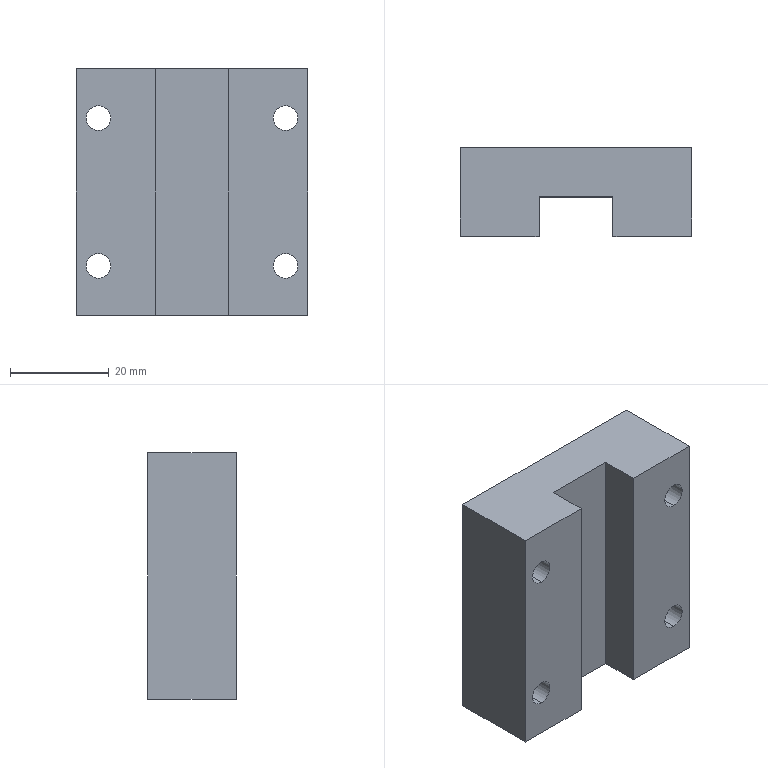Part | 1 solid | 18 faces | box 47 x 18 x 50 mm | volume 34886 mm3 | plane 10 | cylinder 8 | commonest cylinder face diameters 5 x8
STEP:
#1=CARTESIAN_POINT('',(-19.,-9.,37.5));
#2=VERTEX_POINT('',#1);
#3=CARTESIAN_POINT('',(-19.,-9.,42.5));
#4=VERTEX_POINT('',#3);
#5=CARTESIAN_POINT('',(-19.,-9.,40.));
#6=DIRECTION('',(0.,1.,0.));
#7=DIRECTION('',(-1.,0.,0.));
#8=AXIS2_PLACEMENT_3D('',#5,#6,#7);
#9=CIRCLE('',#8,2.5);
#10=EDGE_CURVE('',#2,#4,#9,.T.);
#11=ORIENTED_EDGE('',*,*,#10,.F.);
#12=CARTESIAN_POINT('',(-19.,9.,37.5));
#13=VERTEX_POINT('',#12);
#14=CARTESIAN_POINT('',(-19.,-41.,37.5));
#15=DIRECTION('',(0.,1.,0.));
#16=VECTOR('',#15,1000.);
#17=LINE('',#14,#16);
#18=EDGE_CURVE('',#2,#13,#17,.T.);
#19=ORIENTED_EDGE('',*,*,#18,.T.);
#20=CARTESIAN_POINT('',(-19.,9.,42.5));
#21=VERTEX_POINT('',#20);
#22=CARTESIAN_POINT('',(-19.,9.,40.));
#23=DIRECTION('',(0.,1.,0.));
#24=DIRECTION('',(0.,0.,1.));
#25=AXIS2_PLACEMENT_3D('',#22,#23,#24);
#26=CIRCLE('',#25,2.5);
#27=EDGE_CURVE('',#13,#21,#26,.T.);
#28=ORIENTED_EDGE('',*,*,#27,.T.);
#29=CARTESIAN_POINT('',(-19.,-41.,42.5));
#30=DIRECTION('',(0.,1.,0.));
#31=VECTOR('',#30,1000.);
#32=LINE('',#29,#31);
#33=EDGE_CURVE('',#4,#21,#32,.T.);
#34=ORIENTED_EDGE('',*,*,#33,.F.);
#35=EDGE_LOOP('',(#11,#19,#28,#34));
#36=FACE_OUTER_BOUND('',#35,.T.);
#37=CARTESIAN_POINT('',(-19.,-41.,40.));
#38=DIRECTION('',(0.,1.,0.));
#39=DIRECTION('',(0.,0.,1.));
#40=AXIS2_PLACEMENT_3D('',#37,#38,#39);
#41=CYLINDRICAL_SURFACE('',#40,2.5);
#42=ADVANCED_FACE('',(#36),#41,.F.);
#43=CARTESIAN_POINT('',(-19.,-9.,7.5));
#44=VERTEX_POINT('',#43);
#45=CARTESIAN_POINT('',(-19.,-9.,12.5));
#46=VERTEX_POINT('',#45);
#47=CARTESIAN_POINT('',(-19.,-9.,10.));
#48=DIRECTION('',(0.,1.,0.));
#49=DIRECTION('',(-1.,0.,0.));
#50=AXIS2_PLACEMENT_3D('',#47,#48,#49);
#51=CIRCLE('',#50,2.5);
#52=EDGE_CURVE('',#44,#46,#51,.T.);
#53=ORIENTED_EDGE('',*,*,#52,.F.);
#54=CARTESIAN_POINT('',(-19.,9.,7.5));
#55=VERTEX_POINT('',#54);
#56=CARTESIAN_POINT('',(-19.,-41.,7.5));
#57=DIRECTION('',(0.,1.,0.));
#58=VECTOR('',#57,1000.);
#59=LINE('',#56,#58);
#60=EDGE_CURVE('',#44,#55,#59,.T.);
#61=ORIENTED_EDGE('',*,*,#60,.T.);
#62=CARTESIAN_POINT('',(-19.,9.,12.5));
#63=VERTEX_POINT('',#62);
#64=CARTESIAN_POINT('',(-19.,9.,10.));
#65=DIRECTION('',(0.,1.,0.));
#66=DIRECTION('',(0.,0.,1.));
#67=AXIS2_PLACEMENT_3D('',#64,#65,#66);
#68=CIRCLE('',#67,2.5);
#69=EDGE_CURVE('',#55,#63,#68,.T.);
#70=ORIENTED_EDGE('',*,*,#69,.T.);
#71=CARTESIAN_POINT('',(-19.,-41.,12.5));
#72=DIRECTION('',(0.,1.,0.));
#73=VECTOR('',#72,1000.);
#74=LINE('',#71,#73);
#75=EDGE_CURVE('',#46,#63,#74,.T.);
#76=ORIENTED_EDGE('',*,*,#75,.F.);
#77=EDGE_LOOP('',(#53,#61,#70,#76));
#78=FACE_OUTER_BOUND('',#77,.T.);
#79=CARTESIAN_POINT('',(-19.,-41.,10.));
#80=DIRECTION('',(0.,1.,0.));
#81=DIRECTION('',(0.,0.,1.));
#82=AXIS2_PLACEMENT_3D('',#79,#80,#81);
#83=CYLINDRICAL_SURFACE('',#82,2.5);
#84=ADVANCED_FACE('',(#78),#83,.F.);
#85=CARTESIAN_POINT('',(19.,-9.,37.5));
#86=VERTEX_POINT('',#85);
#87=CARTESIAN_POINT('',(19.,-9.,42.5));
#88=VERTEX_POINT('',#87);
#89=CARTESIAN_POINT('',(19.,-9.,40.));
#90=DIRECTION('',(0.,1.,0.));
#91=DIRECTION('',(-1.,0.,0.));
#92=AXIS2_PLACEMENT_3D('',#89,#90,#91);
#93=CIRCLE('',#92,2.5);
#94=EDGE_CURVE('',#86,#88,#93,.T.);
#95=ORIENTED_EDGE('',*,*,#94,.F.);
#96=CARTESIAN_POINT('',(19.,9.,37.5));
#97=VERTEX_POINT('',#96);
#98=CARTESIAN_POINT('',(19.,-41.,37.5));
#99=DIRECTION('',(0.,1.,0.));
#100=VECTOR('',#99,1000.);
#101=LINE('',#98,#100);
#102=EDGE_CURVE('',#86,#97,#101,.T.);
#103=ORIENTED_EDGE('',*,*,#102,.T.);
#104=CARTESIAN_POINT('',(19.,9.,42.5));
#105=VERTEX_POINT('',#104);
#106=CARTESIAN_POINT('',(19.,9.,40.));
#107=DIRECTION('',(0.,1.,0.));
#108=DIRECTION('',(0.,0.,1.));
#109=AXIS2_PLACEMENT_3D('',#106,#107,#108);
#110=CIRCLE('',#109,2.5);
#111=EDGE_CURVE('',#97,#105,#110,.T.);
#112=ORIENTED_EDGE('',*,*,#111,.T.);
#113=CARTESIAN_POINT('',(19.,-41.,42.5));
#114=DIRECTION('',(0.,1.,0.));
#115=VECTOR('',#114,1000.);
#116=LINE('',#113,#115);
#117=EDGE_CURVE('',#88,#105,#116,.T.);
#118=ORIENTED_EDGE('',*,*,#117,.F.);
#119=EDGE_LOOP('',(#95,#103,#112,#118));
#120=FACE_OUTER_BOUND('',#119,.T.);
#121=CARTESIAN_POINT('',(19.,-41.,40.));
#122=DIRECTION('',(0.,1.,0.));
#123=DIRECTION('',(0.,0.,1.));
#124=AXIS2_PLACEMENT_3D('',#121,#122,#123);
#125=CYLINDRICAL_SURFACE('',#124,2.5);
#126=ADVANCED_FACE('',(#120),#125,.F.);
#127=CARTESIAN_POINT('',(19.,-9.,7.5));
#128=VERTEX_POINT('',#127);
#129=CARTESIAN_POINT('',(19.,-9.,12.5));
#130=VERTEX_POINT('',#129);
#131=CARTESIAN_POINT('',(19.,-9.,10.));
#132=DIRECTION('',(0.,1.,0.));
#133=DIRECTION('',(-1.,0.,0.));
#134=AXIS2_PLACEMENT_3D('',#131,#132,#133);
#135=CIRCLE('',#134,2.5);
#136=EDGE_CURVE('',#128,#130,#135,.T.);
#137=ORIENTED_EDGE('',*,*,#136,.F.);
#138=CARTESIAN_POINT('',(19.,9.,7.5));
#139=VERTEX_POINT('',#138);
#140=CARTESIAN_POINT('',(19.,-41.,7.5));
#141=DIRECTION('',(0.,1.,0.));
#142=VECTOR('',#141,1000.);
#143=LINE('',#140,#142);
#144=EDGE_CURVE('',#128,#139,#143,.T.);
#145=ORIENTED_EDGE('',*,*,#144,.T.);
#146=CARTESIAN_POINT('',(19.,9.,12.5));
#147=VERTEX_POINT('',#146);
#148=CARTESIAN_POINT('',(19.,9.,10.));
#149=DIRECTION('',(0.,1.,0.));
#150=DIRECTION('',(0.,0.,1.));
#151=AXIS2_PLACEMENT_3D('',#148,#149,#150);
#152=CIRCLE('',#151,2.5);
#153=EDGE_CURVE('',#139,#147,#152,.T.);
#154=ORIENTED_EDGE('',*,*,#153,.T.);
#155=CARTESIAN_POINT('',(19.,-41.,12.5));
#156=DIRECTION('',(0.,1.,0.));
#157=VECTOR('',#156,1000.);
#158=LINE('',#155,#157);
#159=EDGE_CURVE('',#130,#147,#158,.T.);
#160=ORIENTED_EDGE('',*,*,#159,.F.);
#161=EDGE_LOOP('',(#137,#145,#154,#160));
#162=FACE_OUTER_BOUND('',#161,.T.);
#163=CARTESIAN_POINT('',(19.,-41.,10.));
#164=DIRECTION('',(0.,1.,0.));
#165=DIRECTION('',(0.,0.,1.));
#166=AXIS2_PLACEMENT_3D('',#163,#164,#165);
#167=CYLINDRICAL_SURFACE('',#166,2.5);
#168=ADVANCED_FACE('',(#162),#167,.F.);
#169=CARTESIAN_POINT('',(23.5,-9.,0.));
#170=VERTEX_POINT('',#169);
#171=CARTESIAN_POINT('',(23.5,9.,0.));
#172=VERTEX_POINT('',#171);
#173=CARTESIAN_POINT('',(23.5,-9.,0.));
#174=DIRECTION('',(0.,1.,0.));
#175=VECTOR('',#174,1000.);
#176=LINE('',#173,#175);
#177=EDGE_CURVE('',#170,#172,#176,.T.);
#178=ORIENTED_EDGE('',*,*,#177,.T.);
#179=CARTESIAN_POINT('',(23.5,9.,50.));
#180=VERTEX_POINT('',#179);
#181=CARTESIAN_POINT('',(23.5,9.,50.));
#182=DIRECTION('',(0.,0.,-1.));
#183=VECTOR('',#182,1000.);
#184=LINE('',#181,#183);
#185=EDGE_CURVE('',#180,#172,#184,.T.);
#186=ORIENTED_EDGE('',*,*,#185,.F.);
#187=CARTESIAN_POINT('',(23.5,-9.,50.));
#188=VERTEX_POINT('',#187);
#189=CARTESIAN_POINT('',(23.5,-9.,50.));
#190=DIRECTION('',(0.,1.,0.));
#191=VECTOR('',#190,1000.);
#192=LINE('',#189,#191);
#193=EDGE_CURVE('',#188,#180,#192,.T.);
#194=ORIENTED_EDGE('',*,*,#193,.F.);
#195=CARTESIAN_POINT('',(23.5,-9.,50.));
#196=DIRECTION('',(0.,0.,-1.));
#197=VECTOR('',#196,1000.);
#198=LINE('',#195,#197);
#199=EDGE_CURVE('',#188,#170,#198,.T.);
#200=ORIENTED_EDGE('',*,*,#199,.T.);
#201=EDGE_LOOP('',(#178,#186,#194,#200));
#202=FACE_OUTER_BOUND('',#201,.T.);
#203=CARTESIAN_POINT('',(23.5,-9.,50.));
#204=DIRECTION('',(-1.,0.,0.));
#205=DIRECTION('',(0.,0.,1.));
#206=AXIS2_PLACEMENT_3D('',#203,#204,#205);
#207=PLANE('',#206);
#208=ADVANCED_FACE('',(#202),#207,.F.);
#209=CARTESIAN_POINT('',(-19.,9.,40.));
#210=DIRECTION('',(0.,1.,0.));
#211=DIRECTION('',(0.,0.,1.));
#212=AXIS2_PLACEMENT_3D('',#209,#210,#211);
#213=CIRCLE('',#212,2.5);
#214=EDGE_CURVE('',#21,#13,#213,.T.);
#215=ORIENTED_EDGE('',*,*,#214,.F.);
#216=ORIENTED_EDGE('',*,*,#27,.F.);
#217=EDGE_LOOP('',(#215,#216));
#218=FACE_BOUND('',#217,.T.);
#219=CARTESIAN_POINT('',(-19.,9.,10.));
#220=DIRECTION('',(0.,1.,0.));
#221=DIRECTION('',(0.,0.,1.));
#222=AXIS2_PLACEMENT_3D('',#219,#220,#221);
#223=CIRCLE('',#222,2.5);
#224=EDGE_CURVE('',#63,#55,#223,.T.);
#225=ORIENTED_EDGE('',*,*,#224,.F.);
#226=ORIENTED_EDGE('',*,*,#69,.F.);
#227=EDGE_LOOP('',(#225,#226));
#228=FACE_BOUND('',#227,.T.);
#229=CARTESIAN_POINT('',(19.,9.,40.));
#230=DIRECTION('',(0.,1.,0.));
#231=DIRECTION('',(0.,0.,1.));
#232=AXIS2_PLACEMENT_3D('',#229,#230,#231);
#233=CIRCLE('',#232,2.5);
#234=EDGE_CURVE('',#105,#97,#233,.T.);
#235=ORIENTED_EDGE('',*,*,#234,.F.);
#236=ORIENTED_EDGE('',*,*,#111,.F.);
#237=EDGE_LOOP('',(#235,#236));
#238=FACE_BOUND('',#237,.T.);
#239=CARTESIAN_POINT('',(19.,9.,10.));
#240=DIRECTION('',(0.,1.,0.));
#241=DIRECTION('',(0.,0.,1.));
#242=AXIS2_PLACEMENT_3D('',#239,#240,#241);
#243=CIRCLE('',#242,2.5);
#244=EDGE_CURVE('',#147,#139,#243,.T.);
#245=ORIENTED_EDGE('',*,*,#244,.F.);
#246=ORIENTED_EDGE('',*,*,#153,.F.);
#247=EDGE_LOOP('',(#245,#246));
#248=FACE_BOUND('',#247,.T.);
#249=CARTESIAN_POINT('',(-23.5,9.,0.));
#250=VERTEX_POINT('',#249);
#251=CARTESIAN_POINT('',(-23.5,9.,0.));
#252=DIRECTION('',(-1.,0.,0.));
#253=VECTOR('',#252,1000.);
#254=LINE('',#251,#253);
#255=EDGE_CURVE('',#172,#250,#254,.T.);
#256=ORIENTED_EDGE('',*,*,#255,.T.);
#257=CARTESIAN_POINT('',(-23.5,9.,50.));
#258=VERTEX_POINT('',#257);
#259=CARTESIAN_POINT('',(-23.5,9.,50.));
#260=DIRECTION('',(0.,0.,-1.));
#261=VECTOR('',#260,1000.);
#262=LINE('',#259,#261);
#263=EDGE_CURVE('',#258,#250,#262,.T.);
#264=ORIENTED_EDGE('',*,*,#263,.F.);
#265=CARTESIAN_POINT('',(-23.5,9.,50.));
#266=DIRECTION('',(-1.,0.,0.));
#267=VECTOR('',#266,1000.);
#268=LINE('',#265,#267);
#269=EDGE_CURVE('',#180,#258,#268,.T.);
#270=ORIENTED_EDGE('',*,*,#269,.F.);
#271=ORIENTED_EDGE('',*,*,#185,.T.);
#272=EDGE_LOOP('',(#256,#264,#270,#271));
#273=FACE_OUTER_BOUND('',#272,.T.);
#274=CARTESIAN_POINT('',(-23.5,9.,50.));
#275=DIRECTION('',(0.,-1.,0.));
#276=DIRECTION('',(0.,0.,-1.));
#277=AXIS2_PLACEMENT_3D('',#274,#275,#276);
#278=PLANE('',#277);
#279=ADVANCED_FACE('',(#218,#228,#238,#248,#273),#278,.F.);
#280=CARTESIAN_POINT('',(-23.5,-9.,0.));
#281=VERTEX_POINT('',#280);
#282=CARTESIAN_POINT('',(-23.5,-9.,0.));
#283=DIRECTION('',(0.,-1.,0.));
#284=VECTOR('',#283,1000.);
#285=LINE('',#282,#284);
#286=EDGE_CURVE('',#250,#281,#285,.T.);
#287=ORIENTED_EDGE('',*,*,#286,.T.);
#288=CARTESIAN_POINT('',(-23.5,-9.,50.));
#289=VERTEX_POINT('',#288);
#290=CARTESIAN_POINT('',(-23.5,-9.,50.));
#291=DIRECTION('',(0.,0.,-1.));
#292=VECTOR('',#291,1000.);
#293=LINE('',#290,#292);
#294=EDGE_CURVE('',#289,#281,#293,.T.);
#295=ORIENTED_EDGE('',*,*,#294,.F.);
#296=CARTESIAN_POINT('',(-23.5,-9.,50.));
#297=DIRECTION('',(0.,-1.,0.));
#298=VECTOR('',#297,1000.);
#299=LINE('',#296,#298);
#300=EDGE_CURVE('',#258,#289,#299,.T.);
#301=ORIENTED_EDGE('',*,*,#300,.F.);
#302=ORIENTED_EDGE('',*,*,#263,.T.);
#303=EDGE_LOOP('',(#287,#295,#301,#302));
#304=FACE_OUTER_BOUND('',#303,.T.);
#305=CARTESIAN_POINT('',(-23.5,-9.,50.));
#306=DIRECTION('',(1.,0.,0.));
#307=DIRECTION('',(0.,0.,-1.));
#308=AXIS2_PLACEMENT_3D('',#305,#306,#307);
#309=PLANE('',#308);
#310=ADVANCED_FACE('',(#304),#309,.F.);
#311=CARTESIAN_POINT('',(-19.,-9.,40.));
#312=DIRECTION('',(0.,1.,0.));
#313=DIRECTION('',(-1.,0.,0.));
#314=AXIS2_PLACEMENT_3D('',#311,#312,#313);
#315=CIRCLE('',#314,2.5);
#316=EDGE_CURVE('',#4,#2,#315,.T.);
#317=ORIENTED_EDGE('',*,*,#316,.T.);
#318=ORIENTED_EDGE('',*,*,#10,.T.);
#319=EDGE_LOOP('',(#317,#318));
#320=FACE_BOUND('',#319,.T.);
#321=CARTESIAN_POINT('',(-19.,-9.,10.));
#322=DIRECTION('',(0.,1.,0.));
#323=DIRECTION('',(-1.,0.,0.));
#324=AXIS2_PLACEMENT_3D('',#321,#322,#323);
#325=CIRCLE('',#324,2.5);
#326=EDGE_CURVE('',#46,#44,#325,.T.);
#327=ORIENTED_EDGE('',*,*,#326,.T.);
#328=ORIENTED_EDGE('',*,*,#52,.T.);
#329=EDGE_LOOP('',(#327,#328));
#330=FACE_BOUND('',#329,.T.);
#331=CARTESIAN_POINT('',(-7.5,-9.,0.));
#332=VERTEX_POINT('',#331);
#333=CARTESIAN_POINT('',(-23.5,-9.,0.));
#334=DIRECTION('',(1.,0.,0.));
#335=VECTOR('',#334,1000.);
#336=LINE('',#333,#335);
#337=EDGE_CURVE('',#281,#332,#336,.T.);
#338=ORIENTED_EDGE('',*,*,#337,.T.);
#339=CARTESIAN_POINT('',(-7.5,-9.,50.));
#340=VERTEX_POINT('',#339);
#341=CARTESIAN_POINT('',(-7.5,-9.,50.));
#342=DIRECTION('',(0.,0.,-1.));
#343=VECTOR('',#342,1000.);
#344=LINE('',#341,#343);
#345=EDGE_CURVE('',#340,#332,#344,.T.);
#346=ORIENTED_EDGE('',*,*,#345,.F.);
#347=CARTESIAN_POINT('',(-23.5,-9.,50.));
#348=DIRECTION('',(1.,0.,0.));
#349=VECTOR('',#348,1000.);
#350=LINE('',#347,#349);
#351=EDGE_CURVE('',#289,#340,#350,.T.);
#352=ORIENTED_EDGE('',*,*,#351,.F.);
#353=ORIENTED_EDGE('',*,*,#294,.T.);
#354=EDGE_LOOP('',(#338,#346,#352,#353));
#355=FACE_OUTER_BOUND('',#354,.T.);
#356=CARTESIAN_POINT('',(-23.5,-9.,50.));
#357=DIRECTION('',(0.,1.,0.));
#358=DIRECTION('',(-1.,0.,0.));
#359=AXIS2_PLACEMENT_3D('',#356,#357,#358);
#360=PLANE('',#359);
#361=ADVANCED_FACE('',(#320,#330,#355),#360,.F.);
#362=CARTESIAN_POINT('',(-7.5,-1.,0.));
#363=VERTEX_POINT('',#362);
#364=CARTESIAN_POINT('',(-7.5,-9.,0.));
#365=DIRECTION('',(0.,1.,0.));
#366=VECTOR('',#365,1000.);
#367=LINE('',#364,#366);
#368=EDGE_CURVE('',#332,#363,#367,.T.);
#369=ORIENTED_EDGE('',*,*,#368,.T.);
#370=CARTESIAN_POINT('',(-7.5,-1.,50.));
#371=VERTEX_POINT('',#370);
#372=CARTESIAN_POINT('',(-7.5,-1.,50.));
#373=DIRECTION('',(0.,0.,-1.));
#374=VECTOR('',#373,1000.);
#375=LINE('',#372,#374);
#376=EDGE_CURVE('',#371,#363,#375,.T.);
#377=ORIENTED_EDGE('',*,*,#376,.F.);
#378=CARTESIAN_POINT('',(-7.5,-9.,50.));
#379=DIRECTION('',(0.,1.,0.));
#380=VECTOR('',#379,1000.);
#381=LINE('',#378,#380);
#382=EDGE_CURVE('',#340,#371,#381,.T.);
#383=ORIENTED_EDGE('',*,*,#382,.F.);
#384=ORIENTED_EDGE('',*,*,#345,.T.);
#385=EDGE_LOOP('',(#369,#377,#383,#384));
#386=FACE_OUTER_BOUND('',#385,.T.);
#387=CARTESIAN_POINT('',(-7.5,-9.,50.));
#388=DIRECTION('',(-1.,0.,0.));
#389=DIRECTION('',(0.,-1.,0.));
#390=AXIS2_PLACEMENT_3D('',#387,#388,#389);
#391=PLANE('',#390);
#392=ADVANCED_FACE('',(#386),#391,.F.);
#393=CARTESIAN_POINT('',(7.5,-1.,0.));
#394=VERTEX_POINT('',#393);
#395=CARTESIAN_POINT('',(-7.5,-1.,0.));
#396=DIRECTION('',(1.,0.,0.));
#397=VECTOR('',#396,1000.);
#398=LINE('',#395,#397);
#399=EDGE_CURVE('',#363,#394,#398,.T.);
#400=ORIENTED_EDGE('',*,*,#399,.T.);
#401=CARTESIAN_POINT('',(7.5,-1.,50.));
#402=VERTEX_POINT('',#401);
#403=CARTESIAN_POINT('',(7.5,-1.,50.));
#404=DIRECTION('',(0.,0.,-1.));
#405=VECTOR('',#404,1000.);
#406=LINE('',#403,#405);
#407=EDGE_CURVE('',#402,#394,#406,.T.);
#408=ORIENTED_EDGE('',*,*,#407,.F.);
#409=CARTESIAN_POINT('',(-7.5,-1.,50.));
#410=DIRECTION('',(1.,0.,0.));
#411=VECTOR('',#410,1000.);
#412=LINE('',#409,#411);
#413=EDGE_CURVE('',#371,#402,#412,.T.);
#414=ORIENTED_EDGE('',*,*,#413,.F.);
#415=ORIENTED_EDGE('',*,*,#376,.T.);
#416=EDGE_LOOP('',(#400,#408,#414,#415));
#417=FACE_OUTER_BOUND('',#416,.T.);
#418=CARTESIAN_POINT('',(-7.5,-1.,50.));
#419=DIRECTION('',(0.,1.,0.));
#420=DIRECTION('',(-1.,0.,0.));
#421=AXIS2_PLACEMENT_3D('',#418,#419,#420);
#422=PLANE('',#421);
#423=ADVANCED_FACE('',(#417),#422,.F.);
#424=CARTESIAN_POINT('',(7.5,-9.,0.));
#425=VERTEX_POINT('',#424);
#426=CARTESIAN_POINT('',(7.5,-9.,0.));
#427=DIRECTION('',(0.,-1.,0.));
#428=VECTOR('',#427,1000.);
#429=LINE('',#426,#428);
#430=EDGE_CURVE('',#394,#425,#429,.T.);
#431=ORIENTED_EDGE('',*,*,#430,.T.);
#432=CARTESIAN_POINT('',(7.5,-9.,50.));
#433=VERTEX_POINT('',#432);
#434=CARTESIAN_POINT('',(7.5,-9.,50.));
#435=DIRECTION('',(0.,0.,-1.));
#436=VECTOR('',#435,1000.);
#437=LINE('',#434,#436);
#438=EDGE_CURVE('',#433,#425,#437,.T.);
#439=ORIENTED_EDGE('',*,*,#438,.F.);
#440=CARTESIAN_POINT('',(7.5,-9.,50.));
#441=DIRECTION('',(0.,-1.,0.));
#442=VECTOR('',#441,1000.);
#443=LINE('',#440,#442);
#444=EDGE_CURVE('',#402,#433,#443,.T.);
#445=ORIENTED_EDGE('',*,*,#444,.F.);
#446=ORIENTED_EDGE('',*,*,#407,.T.);
#447=EDGE_LOOP('',(#431,#439,#445,#446));
#448=FACE_OUTER_BOUND('',#447,.T.);
#449=CARTESIAN_POINT('',(7.5,-9.,50.));
#450=DIRECTION('',(1.,0.,0.));
#451=DIRECTION('',(0.,1.,0.));
#452=AXIS2_PLACEMENT_3D('',#449,#450,#451);
#453=PLANE('',#452);
#454=ADVANCED_FACE('',(#448),#453,.F.);
#455=CARTESIAN_POINT('',(19.,-9.,40.));
#456=DIRECTION('',(0.,1.,0.));
#457=DIRECTION('',(-1.,0.,0.));
#458=AXIS2_PLACEMENT_3D('',#455,#456,#457);
#459=CIRCLE('',#458,2.5);
#460=EDGE_CURVE('',#88,#86,#459,.T.);
#461=ORIENTED_EDGE('',*,*,#460,.T.);
#462=ORIENTED_EDGE('',*,*,#94,.T.);
#463=EDGE_LOOP('',(#461,#462));
#464=FACE_BOUND('',#463,.T.);
#465=CARTESIAN_POINT('',(19.,-9.,10.));
#466=DIRECTION('',(0.,1.,0.));
#467=DIRECTION('',(-1.,0.,0.));
#468=AXIS2_PLACEMENT_3D('',#465,#466,#467);
#469=CIRCLE('',#468,2.5);
#470=EDGE_CURVE('',#130,#128,#469,.T.);
#471=ORIENTED_EDGE('',*,*,#470,.T.);
#472=ORIENTED_EDGE('',*,*,#136,.T.);
#473=EDGE_LOOP('',(#471,#472));
#474=FACE_BOUND('',#473,.T.);
#475=CARTESIAN_POINT('',(7.5,-9.,0.));
#476=DIRECTION('',(1.,0.,0.));
#477=VECTOR('',#476,1000.);
#478=LINE('',#475,#477);
#479=EDGE_CURVE('',#425,#170,#478,.T.);
#480=ORIENTED_EDGE('',*,*,#479,.T.);
#481=ORIENTED_EDGE('',*,*,#199,.F.);
#482=CARTESIAN_POINT('',(7.5,-9.,50.));
#483=DIRECTION('',(1.,0.,0.));
#484=VECTOR('',#483,1000.);
#485=LINE('',#482,#484);
#486=EDGE_CURVE('',#433,#188,#485,.T.);
#487=ORIENTED_EDGE('',*,*,#486,.F.);
#488=ORIENTED_EDGE('',*,*,#438,.T.);
#489=EDGE_LOOP('',(#480,#481,#487,#488));
#490=FACE_OUTER_BOUND('',#489,.T.);
#491=CARTESIAN_POINT('',(7.5,-9.,50.));
#492=DIRECTION('',(0.,1.,0.));
#493=DIRECTION('',(-1.,0.,0.));
#494=AXIS2_PLACEMENT_3D('',#491,#492,#493);
#495=PLANE('',#494);
#496=ADVANCED_FACE('',(#464,#474,#490),#495,.F.);
#497=ORIENTED_EDGE('',*,*,#193,.T.);
#498=ORIENTED_EDGE('',*,*,#269,.T.);
#499=ORIENTED_EDGE('',*,*,#300,.T.);
#500=ORIENTED_EDGE('',*,*,#351,.T.);
#501=ORIENTED_EDGE('',*,*,#382,.T.);
#502=ORIENTED_EDGE('',*,*,#413,.T.);
#503=ORIENTED_EDGE('',*,*,#444,.T.);
#504=ORIENTED_EDGE('',*,*,#486,.T.);
#505=EDGE_LOOP('',(#497,#498,#499,#500,#501,#502,#503,#504));
#506=FACE_OUTER_BOUND('',#505,.T.);
#507=CARTESIAN_POINT('',(0.,0.,50.));
#508=DIRECTION('',(0.,0.,-1.));
#509=DIRECTION('',(-1.,0.,0.));
#510=AXIS2_PLACEMENT_3D('',#507,#508,#509);
#511=PLANE('',#510);
#512=ADVANCED_FACE('',(#506),#511,.F.);
#513=ORIENTED_EDGE('',*,*,#177,.F.);
#514=ORIENTED_EDGE('',*,*,#479,.F.);
#515=ORIENTED_EDGE('',*,*,#430,.F.);
#516=ORIENTED_EDGE('',*,*,#399,.F.);
#517=ORIENTED_EDGE('',*,*,#368,.F.);
#518=ORIENTED_EDGE('',*,*,#337,.F.);
#519=ORIENTED_EDGE('',*,*,#286,.F.);
#520=ORIENTED_EDGE('',*,*,#255,.F.);
#521=EDGE_LOOP('',(#513,#514,#515,#516,#517,#518,#519,#520));
#522=FACE_OUTER_BOUND('',#521,.T.);
#523=CARTESIAN_POINT('',(0.,0.,0.));
#524=DIRECTION('',(0.,0.,-1.));
#525=DIRECTION('',(-1.,0.,0.));
#526=AXIS2_PLACEMENT_3D('',#523,#524,#525);
#527=PLANE('',#526);
#528=ADVANCED_FACE('',(#522),#527,.T.);
#529=ORIENTED_EDGE('',*,*,#144,.F.);
#530=ORIENTED_EDGE('',*,*,#470,.F.);
#531=ORIENTED_EDGE('',*,*,#159,.T.);
#532=ORIENTED_EDGE('',*,*,#244,.T.);
#533=EDGE_LOOP('',(#529,#530,#531,#532));
#534=FACE_OUTER_BOUND('',#533,.T.);
#535=CARTESIAN_POINT('',(19.,-41.,10.));
#536=DIRECTION('',(0.,1.,0.));
#537=DIRECTION('',(0.,0.,1.));
#538=AXIS2_PLACEMENT_3D('',#535,#536,#537);
#539=CYLINDRICAL_SURFACE('',#538,2.5);
#540=ADVANCED_FACE('',(#534),#539,.F.);
#541=ORIENTED_EDGE('',*,*,#102,.F.);
#542=ORIENTED_EDGE('',*,*,#460,.F.);
#543=ORIENTED_EDGE('',*,*,#117,.T.);
#544=ORIENTED_EDGE('',*,*,#234,.T.);
#545=EDGE_LOOP('',(#541,#542,#543,#544));
#546=FACE_OUTER_BOUND('',#545,.T.);
#547=CARTESIAN_POINT('',(19.,-41.,40.));
#548=DIRECTION('',(0.,1.,0.));
#549=DIRECTION('',(0.,0.,1.));
#550=AXIS2_PLACEMENT_3D('',#547,#548,#549);
#551=CYLINDRICAL_SURFACE('',#550,2.5);
#552=ADVANCED_FACE('',(#546),#551,.F.);
#553=ORIENTED_EDGE('',*,*,#60,.F.);
#554=ORIENTED_EDGE('',*,*,#326,.F.);
#555=ORIENTED_EDGE('',*,*,#75,.T.);
#556=ORIENTED_EDGE('',*,*,#224,.T.);
#557=EDGE_LOOP('',(#553,#554,#555,#556));
#558=FACE_OUTER_BOUND('',#557,.T.);
#559=CARTESIAN_POINT('',(-19.,-41.,10.));
#560=DIRECTION('',(0.,1.,0.));
#561=DIRECTION('',(0.,0.,1.));
#562=AXIS2_PLACEMENT_3D('',#559,#560,#561);
#563=CYLINDRICAL_SURFACE('',#562,2.5);
#564=ADVANCED_FACE('',(#558),#563,.F.);
#565=ORIENTED_EDGE('',*,*,#18,.F.);
#566=ORIENTED_EDGE('',*,*,#316,.F.);
#567=ORIENTED_EDGE('',*,*,#33,.T.);
#568=ORIENTED_EDGE('',*,*,#214,.T.);
#569=EDGE_LOOP('',(#565,#566,#567,#568));
#570=FACE_OUTER_BOUND('',#569,.T.);
#571=CARTESIAN_POINT('',(-19.,-41.,40.));
#572=DIRECTION('',(0.,1.,0.));
#573=DIRECTION('',(0.,0.,1.));
#574=AXIS2_PLACEMENT_3D('',#571,#572,#573);
#575=CYLINDRICAL_SURFACE('',#574,2.5);
#576=ADVANCED_FACE('',(#570),#575,.F.);
#577=CLOSED_SHELL('',(#42,#84,#126,#168,#208,#279,#310,#361,#392,#423,#454,#496,#512,#528,#540,#552,#564,#576));
#578=MANIFOLD_SOLID_BREP('',#577);
#579=CARTESIAN_POINT('',(0.,0.,0.));
#580=DIRECTION('',(0.,0.,1.));
#581=DIRECTION('',(1.,0.,0.));
#582=AXIS2_PLACEMENT_3D('',#579,#580,#581);
#583=(LENGTH_UNIT()NAMED_UNIT(*)SI_UNIT(.MILLI.,.METRE.));
#584=UNCERTAINTY_MEASURE_WITH_UNIT(LENGTH_MEASURE(0.00001),#583,'','');
#585=(NAMED_UNIT(*)PLANE_ANGLE_UNIT()SI_UNIT($,.RADIAN.));
#586=(NAMED_UNIT(*)SI_UNIT($,.STERADIAN.)SOLID_ANGLE_UNIT());
#587=(GEOMETRIC_REPRESENTATION_CONTEXT(3)GLOBAL_UNCERTAINTY_ASSIGNED_CONTEXT((#584))GLOBAL_UNIT_ASSIGNED_CONTEXT((#583,#585,#586))REPRESENTATION_CONTEXT('',''));
#588=ADVANCED_BREP_SHAPE_REPRESENTATION('',(#578,#582),#587);